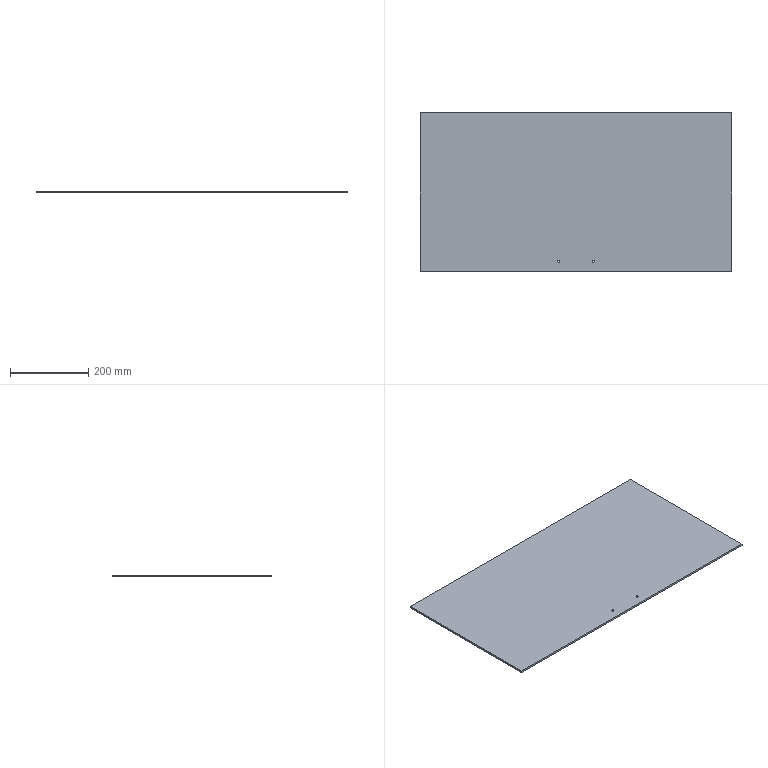Part | SolidWorks | features BaseBody 1 | 1 solid | 10 faces | box 796 x 405 x 5 mm | volume 1611704 mm3 | plane 6 | cylinder 4 | commonest cylinder face diameters 5 x4
STEP:
#1=CARTESIAN_POINT('',(-354.,27.5,5.));
#2=VERTEX_POINT('',#1);
#3=CARTESIAN_POINT('',(-354.,22.5,5.));
#4=VERTEX_POINT('',#3);
#5=CARTESIAN_POINT('',(-354.,25.,5.));
#6=DIRECTION('',(0.,0.,1.));
#7=DIRECTION('',(0.,1.,0.));
#8=AXIS2_PLACEMENT_3D('',#5,#6,#7);
#9=CIRCLE('',#8,2.5);
#10=EDGE_CURVE('',#2,#4,#9,.T.);
#11=ORIENTED_EDGE('',*,*,#10,.T.);
#12=CARTESIAN_POINT('',(-354.,22.5,0.));
#13=VERTEX_POINT('',#12);
#14=CARTESIAN_POINT('',(-354.,22.5,5.));
#15=DIRECTION('',(0.,0.,-1.));
#16=VECTOR('',#15,1000.);
#17=LINE('',#14,#16);
#18=EDGE_CURVE('',#4,#13,#17,.T.);
#19=ORIENTED_EDGE('',*,*,#18,.T.);
#20=CARTESIAN_POINT('',(-354.,27.5,0.));
#21=VERTEX_POINT('',#20);
#22=CARTESIAN_POINT('',(-354.,25.,0.));
#23=DIRECTION('',(0.,0.,-1.));
#24=DIRECTION('',(0.,1.,0.));
#25=AXIS2_PLACEMENT_3D('',#22,#23,#24);
#26=CIRCLE('',#25,2.5);
#27=EDGE_CURVE('',#13,#21,#26,.T.);
#28=ORIENTED_EDGE('',*,*,#27,.T.);
#29=CARTESIAN_POINT('',(-354.,27.5,5.));
#30=DIRECTION('',(0.,0.,-1.));
#31=VECTOR('',#30,1000.);
#32=LINE('',#29,#31);
#33=EDGE_CURVE('',#2,#21,#32,.T.);
#34=ORIENTED_EDGE('',*,*,#33,.F.);
#35=EDGE_LOOP('',(#11,#19,#28,#34));
#36=FACE_OUTER_BOUND('',#35,.T.);
#37=CARTESIAN_POINT('',(-354.,25.,5.));
#38=DIRECTION('',(0.,0.,-1.));
#39=DIRECTION('',(0.,1.,0.));
#40=AXIS2_PLACEMENT_3D('',#37,#38,#39);
#41=CYLINDRICAL_SURFACE('',#40,2.5);
#42=ADVANCED_FACE('',(#36),#41,.F.);
#43=CARTESIAN_POINT('',(-442.,22.5,5.));
#44=VERTEX_POINT('',#43);
#45=CARTESIAN_POINT('',(-442.,27.5,5.));
#46=VERTEX_POINT('',#45);
#47=CARTESIAN_POINT('',(-442.,25.,5.));
#48=DIRECTION('',(0.,0.,-1.));
#49=DIRECTION('',(0.,1.,0.));
#50=AXIS2_PLACEMENT_3D('',#47,#48,#49);
#51=CIRCLE('',#50,2.5);
#52=EDGE_CURVE('',#44,#46,#51,.T.);
#53=ORIENTED_EDGE('',*,*,#52,.F.);
#54=CARTESIAN_POINT('',(-442.,22.5,0.));
#55=VERTEX_POINT('',#54);
#56=CARTESIAN_POINT('',(-442.,22.5,5.));
#57=DIRECTION('',(0.,0.,-1.));
#58=VECTOR('',#57,1000.);
#59=LINE('',#56,#58);
#60=EDGE_CURVE('',#44,#55,#59,.T.);
#61=ORIENTED_EDGE('',*,*,#60,.T.);
#62=CARTESIAN_POINT('',(-442.,27.5,0.));
#63=VERTEX_POINT('',#62);
#64=CARTESIAN_POINT('',(-442.,25.,0.));
#65=DIRECTION('',(0.,0.,-1.));
#66=DIRECTION('',(0.,1.,0.));
#67=AXIS2_PLACEMENT_3D('',#64,#65,#66);
#68=CIRCLE('',#67,2.5);
#69=EDGE_CURVE('',#55,#63,#68,.T.);
#70=ORIENTED_EDGE('',*,*,#69,.T.);
#71=CARTESIAN_POINT('',(-442.,27.5,5.));
#72=DIRECTION('',(0.,0.,-1.));
#73=VECTOR('',#72,1000.);
#74=LINE('',#71,#73);
#75=EDGE_CURVE('',#46,#63,#74,.T.);
#76=ORIENTED_EDGE('',*,*,#75,.F.);
#77=EDGE_LOOP('',(#53,#61,#70,#76));
#78=FACE_OUTER_BOUND('',#77,.T.);
#79=CARTESIAN_POINT('',(-442.,25.,5.));
#80=DIRECTION('',(0.,0.,-1.));
#81=DIRECTION('',(0.,1.,0.));
#82=AXIS2_PLACEMENT_3D('',#79,#80,#81);
#83=CYLINDRICAL_SURFACE('',#82,2.5);
#84=ADVANCED_FACE('',(#78),#83,.F.);
#85=ORIENTED_EDGE('',*,*,#18,.F.);
#86=CARTESIAN_POINT('',(-354.,25.,5.));
#87=DIRECTION('',(0.,0.,1.));
#88=DIRECTION('',(0.,1.,0.));
#89=AXIS2_PLACEMENT_3D('',#86,#87,#88);
#90=CIRCLE('',#89,2.5);
#91=EDGE_CURVE('',#4,#2,#90,.T.);
#92=ORIENTED_EDGE('',*,*,#91,.T.);
#93=ORIENTED_EDGE('',*,*,#33,.T.);
#94=CARTESIAN_POINT('',(-354.,25.,0.));
#95=DIRECTION('',(0.,0.,-1.));
#96=DIRECTION('',(0.,1.,0.));
#97=AXIS2_PLACEMENT_3D('',#94,#95,#96);
#98=CIRCLE('',#97,2.5);
#99=EDGE_CURVE('',#21,#13,#98,.T.);
#100=ORIENTED_EDGE('',*,*,#99,.T.);
#101=EDGE_LOOP('',(#85,#92,#93,#100));
#102=FACE_OUTER_BOUND('',#101,.T.);
#103=CARTESIAN_POINT('',(-354.,25.,5.));
#104=DIRECTION('',(0.,0.,-1.));
#105=DIRECTION('',(0.,1.,0.));
#106=AXIS2_PLACEMENT_3D('',#103,#104,#105);
#107=CYLINDRICAL_SURFACE('',#106,2.5);
#108=ADVANCED_FACE('',(#102),#107,.F.);
#109=CARTESIAN_POINT('',(-442.,25.,0.));
#110=DIRECTION('',(0.,0.,-1.));
#111=DIRECTION('',(0.,1.,0.));
#112=AXIS2_PLACEMENT_3D('',#109,#110,#111);
#113=CIRCLE('',#112,2.5);
#114=EDGE_CURVE('',#63,#55,#113,.T.);
#115=ORIENTED_EDGE('',*,*,#114,.F.);
#116=ORIENTED_EDGE('',*,*,#69,.F.);
#117=EDGE_LOOP('',(#115,#116));
#118=FACE_BOUND('',#117,.T.);
#119=ORIENTED_EDGE('',*,*,#99,.F.);
#120=ORIENTED_EDGE('',*,*,#27,.F.);
#121=EDGE_LOOP('',(#119,#120));
#122=FACE_BOUND('',#121,.T.);
#123=CARTESIAN_POINT('',(-796.,0.,0.));
#124=VERTEX_POINT('',#123);
#125=CARTESIAN_POINT('',(0.,0.,0.));
#126=VERTEX_POINT('',#125);
#127=CARTESIAN_POINT('',(-398.,0.,0.));
#128=DIRECTION('',(1.,0.,0.));
#129=VECTOR('',#128,1000.);
#130=LINE('',#127,#129);
#131=EDGE_CURVE('',#124,#126,#130,.T.);
#132=ORIENTED_EDGE('',*,*,#131,.F.);
#133=CARTESIAN_POINT('',(-796.,405.,0.));
#134=VERTEX_POINT('',#133);
#135=CARTESIAN_POINT('',(-796.,202.5,0.));
#136=DIRECTION('',(0.,-1.,0.));
#137=VECTOR('',#136,1000.);
#138=LINE('',#135,#137);
#139=EDGE_CURVE('',#134,#124,#138,.T.);
#140=ORIENTED_EDGE('',*,*,#139,.F.);
#141=CARTESIAN_POINT('',(0.,405.,0.));
#142=VERTEX_POINT('',#141);
#143=CARTESIAN_POINT('',(-398.,405.,0.));
#144=DIRECTION('',(-1.,0.,0.));
#145=VECTOR('',#144,1000.);
#146=LINE('',#143,#145);
#147=EDGE_CURVE('',#142,#134,#146,.T.);
#148=ORIENTED_EDGE('',*,*,#147,.F.);
#149=CARTESIAN_POINT('',(0.,202.5,0.));
#150=DIRECTION('',(0.,1.,0.));
#151=VECTOR('',#150,1000.);
#152=LINE('',#149,#151);
#153=EDGE_CURVE('',#126,#142,#152,.T.);
#154=ORIENTED_EDGE('',*,*,#153,.F.);
#155=EDGE_LOOP('',(#132,#140,#148,#154));
#156=FACE_OUTER_BOUND('',#155,.T.);
#157=CARTESIAN_POINT('',(-796.,0.,0.));
#158=DIRECTION('',(0.,0.,1.));
#159=DIRECTION('',(1.,0.,0.));
#160=AXIS2_PLACEMENT_3D('',#157,#158,#159);
#161=PLANE('',#160);
#162=ADVANCED_FACE('',(#118,#122,#156),#161,.F.);
#163=CARTESIAN_POINT('',(-442.,25.,5.));
#164=DIRECTION('',(0.,0.,-1.));
#165=DIRECTION('',(0.,1.,0.));
#166=AXIS2_PLACEMENT_3D('',#163,#164,#165);
#167=CIRCLE('',#166,2.5);
#168=EDGE_CURVE('',#46,#44,#167,.T.);
#169=ORIENTED_EDGE('',*,*,#168,.T.);
#170=ORIENTED_EDGE('',*,*,#52,.T.);
#171=EDGE_LOOP('',(#169,#170));
#172=FACE_BOUND('',#171,.T.);
#173=ORIENTED_EDGE('',*,*,#10,.F.);
#174=ORIENTED_EDGE('',*,*,#91,.F.);
#175=EDGE_LOOP('',(#173,#174));
#176=FACE_BOUND('',#175,.T.);
#177=CARTESIAN_POINT('',(-796.,405.,5.));
#178=VERTEX_POINT('',#177);
#179=CARTESIAN_POINT('',(-796.,0.,5.));
#180=VERTEX_POINT('',#179);
#181=CARTESIAN_POINT('',(-796.,202.5,5.));
#182=DIRECTION('',(0.,-1.,0.));
#183=VECTOR('',#182,1000.);
#184=LINE('',#181,#183);
#185=EDGE_CURVE('',#178,#180,#184,.T.);
#186=ORIENTED_EDGE('',*,*,#185,.T.);
#187=CARTESIAN_POINT('',(0.,0.,5.));
#188=VERTEX_POINT('',#187);
#189=CARTESIAN_POINT('',(-398.,0.,5.));
#190=DIRECTION('',(1.,0.,0.));
#191=VECTOR('',#190,1000.);
#192=LINE('',#189,#191);
#193=EDGE_CURVE('',#180,#188,#192,.T.);
#194=ORIENTED_EDGE('',*,*,#193,.T.);
#195=CARTESIAN_POINT('',(0.,405.,5.));
#196=VERTEX_POINT('',#195);
#197=CARTESIAN_POINT('',(0.,202.5,5.));
#198=DIRECTION('',(0.,1.,0.));
#199=VECTOR('',#198,1000.);
#200=LINE('',#197,#199);
#201=EDGE_CURVE('',#188,#196,#200,.T.);
#202=ORIENTED_EDGE('',*,*,#201,.T.);
#203=CARTESIAN_POINT('',(-398.,405.,5.));
#204=DIRECTION('',(-1.,0.,0.));
#205=VECTOR('',#204,1000.);
#206=LINE('',#203,#205);
#207=EDGE_CURVE('',#196,#178,#206,.T.);
#208=ORIENTED_EDGE('',*,*,#207,.T.);
#209=EDGE_LOOP('',(#186,#194,#202,#208));
#210=FACE_OUTER_BOUND('',#209,.T.);
#211=CARTESIAN_POINT('',(-796.,0.,5.));
#212=DIRECTION('',(0.,0.,1.));
#213=DIRECTION('',(1.,0.,0.));
#214=AXIS2_PLACEMENT_3D('',#211,#212,#213);
#215=PLANE('',#214);
#216=ADVANCED_FACE('',(#172,#176,#210),#215,.T.);
#217=ORIENTED_EDGE('',*,*,#60,.F.);
#218=ORIENTED_EDGE('',*,*,#168,.F.);
#219=ORIENTED_EDGE('',*,*,#75,.T.);
#220=ORIENTED_EDGE('',*,*,#114,.T.);
#221=EDGE_LOOP('',(#217,#218,#219,#220));
#222=FACE_OUTER_BOUND('',#221,.T.);
#223=CARTESIAN_POINT('',(-442.,25.,5.));
#224=DIRECTION('',(0.,0.,-1.));
#225=DIRECTION('',(0.,1.,0.));
#226=AXIS2_PLACEMENT_3D('',#223,#224,#225);
#227=CYLINDRICAL_SURFACE('',#226,2.5);
#228=ADVANCED_FACE('',(#222),#227,.F.);
#229=CARTESIAN_POINT('',(0.,405.,2.5));
#230=DIRECTION('',(0.,0.,-1.));
#231=VECTOR('',#230,1000.);
#232=LINE('',#229,#231);
#233=EDGE_CURVE('',#196,#142,#232,.T.);
#234=ORIENTED_EDGE('',*,*,#233,.F.);
#235=ORIENTED_EDGE('',*,*,#201,.F.);
#236=CARTESIAN_POINT('',(0.,0.,2.5));
#237=DIRECTION('',(0.,0.,1.));
#238=VECTOR('',#237,1000.);
#239=LINE('',#236,#238);
#240=EDGE_CURVE('',#126,#188,#239,.T.);
#241=ORIENTED_EDGE('',*,*,#240,.F.);
#242=ORIENTED_EDGE('',*,*,#153,.T.);
#243=EDGE_LOOP('',(#234,#235,#241,#242));
#244=FACE_OUTER_BOUND('',#243,.T.);
#245=CARTESIAN_POINT('',(0.,0.,0.));
#246=DIRECTION('',(-1.,0.,0.));
#247=DIRECTION('',(0.,0.,1.));
#248=AXIS2_PLACEMENT_3D('',#245,#246,#247);
#249=PLANE('',#248);
#250=ADVANCED_FACE('',(#244),#249,.F.);
#251=ORIENTED_EDGE('',*,*,#240,.T.);
#252=ORIENTED_EDGE('',*,*,#193,.F.);
#253=CARTESIAN_POINT('',(-796.,0.,2.5));
#254=DIRECTION('',(0.,0.,1.));
#255=VECTOR('',#254,1000.);
#256=LINE('',#253,#255);
#257=EDGE_CURVE('',#124,#180,#256,.T.);
#258=ORIENTED_EDGE('',*,*,#257,.F.);
#259=ORIENTED_EDGE('',*,*,#131,.T.);
#260=EDGE_LOOP('',(#251,#252,#258,#259));
#261=FACE_OUTER_BOUND('',#260,.T.);
#262=CARTESIAN_POINT('',(0.,0.,0.));
#263=DIRECTION('',(0.,1.,0.));
#264=DIRECTION('',(-1.,0.,0.));
#265=AXIS2_PLACEMENT_3D('',#262,#263,#264);
#266=PLANE('',#265);
#267=ADVANCED_FACE('',(#261),#266,.F.);
#268=ORIENTED_EDGE('',*,*,#257,.T.);
#269=ORIENTED_EDGE('',*,*,#185,.F.);
#270=CARTESIAN_POINT('',(-796.,405.,2.5));
#271=DIRECTION('',(0.,0.,1.));
#272=VECTOR('',#271,1000.);
#273=LINE('',#270,#272);
#274=EDGE_CURVE('',#134,#178,#273,.T.);
#275=ORIENTED_EDGE('',*,*,#274,.F.);
#276=ORIENTED_EDGE('',*,*,#139,.T.);
#277=EDGE_LOOP('',(#268,#269,#275,#276));
#278=FACE_OUTER_BOUND('',#277,.T.);
#279=CARTESIAN_POINT('',(-796.,0.,5.));
#280=DIRECTION('',(1.,0.,0.));
#281=DIRECTION('',(0.,0.,-1.));
#282=AXIS2_PLACEMENT_3D('',#279,#280,#281);
#283=PLANE('',#282);
#284=ADVANCED_FACE('',(#278),#283,.F.);
#285=ORIENTED_EDGE('',*,*,#274,.T.);
#286=ORIENTED_EDGE('',*,*,#207,.F.);
#287=ORIENTED_EDGE('',*,*,#233,.T.);
#288=ORIENTED_EDGE('',*,*,#147,.T.);
#289=EDGE_LOOP('',(#285,#286,#287,#288));
#290=FACE_OUTER_BOUND('',#289,.T.);
#291=CARTESIAN_POINT('',(-796.,405.,0.));
#292=DIRECTION('',(0.,-1.,0.));
#293=DIRECTION('',(1.,0.,0.));
#294=AXIS2_PLACEMENT_3D('',#291,#292,#293);
#295=PLANE('',#294);
#296=ADVANCED_FACE('',(#290),#295,.F.);
#297=CLOSED_SHELL('',(#42,#84,#108,#162,#216,#228,#250,#267,#284,#296));
#298=MANIFOLD_SOLID_BREP('',#297);
#299=CARTESIAN_POINT('',(0.,0.,0.));
#300=DIRECTION('',(0.,0.,1.));
#301=DIRECTION('',(1.,0.,0.));
#302=AXIS2_PLACEMENT_3D('',#299,#300,#301);
#303=(LENGTH_UNIT()NAMED_UNIT(*)SI_UNIT(.MILLI.,.METRE.));
#304=UNCERTAINTY_MEASURE_WITH_UNIT(LENGTH_MEASURE(0.00001),#303,'','');
#305=(NAMED_UNIT(*)PLANE_ANGLE_UNIT()SI_UNIT($,.RADIAN.));
#306=(NAMED_UNIT(*)SI_UNIT($,.STERADIAN.)SOLID_ANGLE_UNIT());
#307=(GEOMETRIC_REPRESENTATION_CONTEXT(3)GLOBAL_UNCERTAINTY_ASSIGNED_CONTEXT((#304))GLOBAL_UNIT_ASSIGNED_CONTEXT((#303,#305,#306))REPRESENTATION_CONTEXT('',''));
#308=ADVANCED_BREP_SHAPE_REPRESENTATION('',(#298,#302),#307);